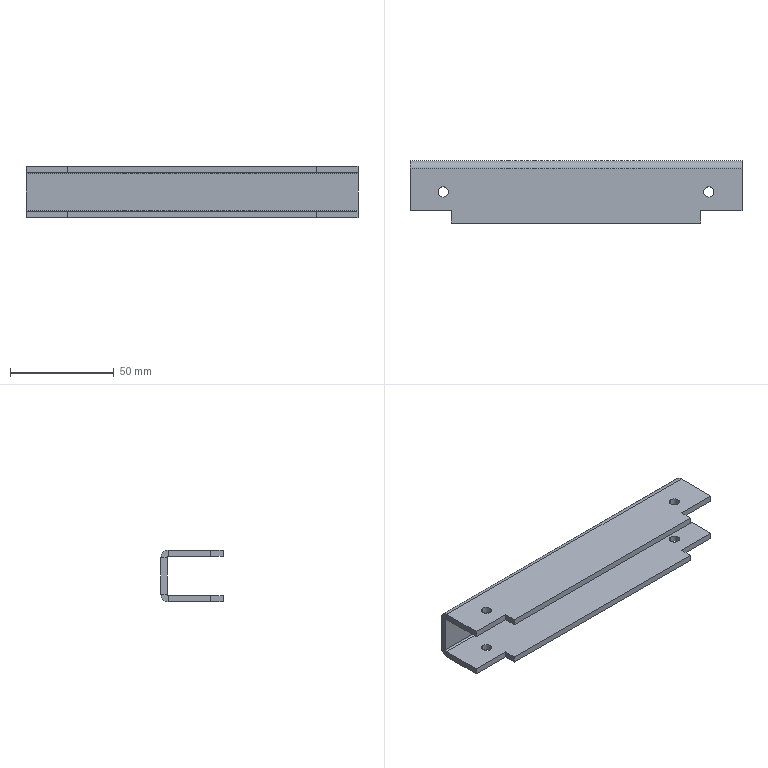Part | SolidWorks | features EdgeFlange 1, Fillet 1, FlatPattern 1, HoleWzd 1, ICE 1, SMBaseFlange 1, SheetMetal 1 | 1 solid | 38 faces | box 160 x 30 x 25 mm | volume 35323 mm3 | plane 26 | cylinder 12 | commonest cylinder face diameters 5 x8 1.473 x2 7.473 x2
STEP:
#1=CARTESIAN_POINT('',(64.,-17.5,12.5));
#2=VERTEX_POINT('',#1);
#3=CARTESIAN_POINT('',(64.,-12.5,12.5));
#4=VERTEX_POINT('',#3);
#5=CARTESIAN_POINT('',(64.,-15.,12.5));
#6=DIRECTION('',(0.,0.,-1.));
#7=DIRECTION('',(0.,1.,0.));
#8=AXIS2_PLACEMENT_3D('',#5,#6,#7);
#9=CIRCLE('',#8,2.5);
#10=EDGE_CURVE('',#2,#4,#9,.T.);
#11=ORIENTED_EDGE('',*,*,#10,.F.);
#12=CARTESIAN_POINT('',(64.,-17.5,9.5));
#13=VERTEX_POINT('',#12);
#14=CARTESIAN_POINT('',(64.,-17.5,-12.5));
#15=DIRECTION('',(0.,0.,-1.));
#16=VECTOR('',#15,1000.);
#17=LINE('',#14,#16);
#18=EDGE_CURVE('',#2,#13,#17,.T.);
#19=ORIENTED_EDGE('',*,*,#18,.T.);
#20=CARTESIAN_POINT('',(64.,-12.5,9.5));
#21=VERTEX_POINT('',#20);
#22=CARTESIAN_POINT('',(64.,-15.,9.5));
#23=DIRECTION('',(0.,0.,-1.));
#24=DIRECTION('',(0.,1.,0.));
#25=AXIS2_PLACEMENT_3D('',#22,#23,#24);
#26=CIRCLE('',#25,2.5);
#27=EDGE_CURVE('',#13,#21,#26,.T.);
#28=ORIENTED_EDGE('',*,*,#27,.T.);
#29=CARTESIAN_POINT('',(64.,-12.5,-12.5));
#30=DIRECTION('',(0.,0.,-1.));
#31=VECTOR('',#30,1000.);
#32=LINE('',#29,#31);
#33=EDGE_CURVE('',#4,#21,#32,.T.);
#34=ORIENTED_EDGE('',*,*,#33,.F.);
#35=EDGE_LOOP('',(#11,#19,#28,#34));
#36=FACE_OUTER_BOUND('',#35,.T.);
#37=CARTESIAN_POINT('',(64.,-15.,-12.5));
#38=DIRECTION('',(0.,0.,-1.));
#39=DIRECTION('',(0.,1.,0.));
#40=AXIS2_PLACEMENT_3D('',#37,#38,#39);
#41=CYLINDRICAL_SURFACE('',#40,2.5);
#42=ADVANCED_FACE('',(#36),#41,.F.);
#43=CARTESIAN_POINT('',(64.,-12.5,-9.5));
#44=VERTEX_POINT('',#43);
#45=CARTESIAN_POINT('',(64.,-17.5,-9.5));
#46=VERTEX_POINT('',#45);
#47=CARTESIAN_POINT('',(64.,-15.,-9.5));
#48=DIRECTION('',(0.,0.,1.));
#49=DIRECTION('',(0.,-1.,0.));
#50=AXIS2_PLACEMENT_3D('',#47,#48,#49);
#51=CIRCLE('',#50,2.5);
#52=EDGE_CURVE('',#44,#46,#51,.T.);
#53=ORIENTED_EDGE('',*,*,#52,.T.);
#54=CARTESIAN_POINT('',(64.,-17.5,-12.5));
#55=VERTEX_POINT('',#54);
#56=CARTESIAN_POINT('',(64.,-17.5,-12.5));
#57=DIRECTION('',(0.,0.,-1.));
#58=VECTOR('',#57,1000.);
#59=LINE('',#56,#58);
#60=EDGE_CURVE('',#46,#55,#59,.T.);
#61=ORIENTED_EDGE('',*,*,#60,.T.);
#62=CARTESIAN_POINT('',(64.,-12.5,-12.5));
#63=VERTEX_POINT('',#62);
#64=CARTESIAN_POINT('',(64.,-15.,-12.5));
#65=DIRECTION('',(0.,0.,-1.));
#66=DIRECTION('',(0.,1.,0.));
#67=AXIS2_PLACEMENT_3D('',#64,#65,#66);
#68=CIRCLE('',#67,2.5);
#69=EDGE_CURVE('',#55,#63,#68,.T.);
#70=ORIENTED_EDGE('',*,*,#69,.T.);
#71=CARTESIAN_POINT('',(64.,-12.5,-12.5));
#72=DIRECTION('',(0.,0.,-1.));
#73=VECTOR('',#72,1000.);
#74=LINE('',#71,#73);
#75=EDGE_CURVE('',#44,#63,#74,.T.);
#76=ORIENTED_EDGE('',*,*,#75,.F.);
#77=EDGE_LOOP('',(#53,#61,#70,#76));
#78=FACE_OUTER_BOUND('',#77,.T.);
#79=CARTESIAN_POINT('',(64.,-15.,-12.5));
#80=DIRECTION('',(0.,0.,-1.));
#81=DIRECTION('',(0.,1.,0.));
#82=AXIS2_PLACEMENT_3D('',#79,#80,#81);
#83=CYLINDRICAL_SURFACE('',#82,2.5);
#84=ADVANCED_FACE('',(#78),#83,.F.);
#85=CARTESIAN_POINT('',(-64.,-17.5,12.5));
#86=VERTEX_POINT('',#85);
#87=CARTESIAN_POINT('',(-64.,-12.5,12.5));
#88=VERTEX_POINT('',#87);
#89=CARTESIAN_POINT('',(-64.,-15.,12.5));
#90=DIRECTION('',(0.,0.,-1.));
#91=DIRECTION('',(0.,1.,0.));
#92=AXIS2_PLACEMENT_3D('',#89,#90,#91);
#93=CIRCLE('',#92,2.5);
#94=EDGE_CURVE('',#86,#88,#93,.T.);
#95=ORIENTED_EDGE('',*,*,#94,.F.);
#96=CARTESIAN_POINT('',(-64.,-17.5,9.5));
#97=VERTEX_POINT('',#96);
#98=CARTESIAN_POINT('',(-64.,-17.5,-12.5));
#99=DIRECTION('',(0.,0.,-1.));
#100=VECTOR('',#99,1000.);
#101=LINE('',#98,#100);
#102=EDGE_CURVE('',#86,#97,#101,.T.);
#103=ORIENTED_EDGE('',*,*,#102,.T.);
#104=CARTESIAN_POINT('',(-64.,-12.5,9.5));
#105=VERTEX_POINT('',#104);
#106=CARTESIAN_POINT('',(-64.,-15.,9.5));
#107=DIRECTION('',(0.,0.,-1.));
#108=DIRECTION('',(0.,1.,0.));
#109=AXIS2_PLACEMENT_3D('',#106,#107,#108);
#110=CIRCLE('',#109,2.5);
#111=EDGE_CURVE('',#97,#105,#110,.T.);
#112=ORIENTED_EDGE('',*,*,#111,.T.);
#113=CARTESIAN_POINT('',(-64.,-12.5,-12.5));
#114=DIRECTION('',(0.,0.,-1.));
#115=VECTOR('',#114,1000.);
#116=LINE('',#113,#115);
#117=EDGE_CURVE('',#88,#105,#116,.T.);
#118=ORIENTED_EDGE('',*,*,#117,.F.);
#119=EDGE_LOOP('',(#95,#103,#112,#118));
#120=FACE_OUTER_BOUND('',#119,.T.);
#121=CARTESIAN_POINT('',(-64.,-15.,-12.5));
#122=DIRECTION('',(0.,0.,-1.));
#123=DIRECTION('',(0.,1.,0.));
#124=AXIS2_PLACEMENT_3D('',#121,#122,#123);
#125=CYLINDRICAL_SURFACE('',#124,2.5);
#126=ADVANCED_FACE('',(#120),#125,.F.);
#127=CARTESIAN_POINT('',(-64.,-12.5,-9.5));
#128=VERTEX_POINT('',#127);
#129=CARTESIAN_POINT('',(-64.,-17.5,-9.5));
#130=VERTEX_POINT('',#129);
#131=CARTESIAN_POINT('',(-64.,-15.,-9.5));
#132=DIRECTION('',(0.,0.,1.));
#133=DIRECTION('',(0.,-1.,0.));
#134=AXIS2_PLACEMENT_3D('',#131,#132,#133);
#135=CIRCLE('',#134,2.5);
#136=EDGE_CURVE('',#128,#130,#135,.T.);
#137=ORIENTED_EDGE('',*,*,#136,.T.);
#138=CARTESIAN_POINT('',(-64.,-17.5,-12.5));
#139=VERTEX_POINT('',#138);
#140=CARTESIAN_POINT('',(-64.,-17.5,-12.5));
#141=DIRECTION('',(0.,0.,-1.));
#142=VECTOR('',#141,1000.);
#143=LINE('',#140,#142);
#144=EDGE_CURVE('',#130,#139,#143,.T.);
#145=ORIENTED_EDGE('',*,*,#144,.T.);
#146=CARTESIAN_POINT('',(-64.,-12.5,-12.5));
#147=VERTEX_POINT('',#146);
#148=CARTESIAN_POINT('',(-64.,-15.,-12.5));
#149=DIRECTION('',(0.,0.,-1.));
#150=DIRECTION('',(0.,1.,0.));
#151=AXIS2_PLACEMENT_3D('',#148,#149,#150);
#152=CIRCLE('',#151,2.5);
#153=EDGE_CURVE('',#139,#147,#152,.T.);
#154=ORIENTED_EDGE('',*,*,#153,.T.);
#155=CARTESIAN_POINT('',(-64.,-12.5,-12.5));
#156=DIRECTION('',(0.,0.,-1.));
#157=VECTOR('',#156,1000.);
#158=LINE('',#155,#157);
#159=EDGE_CURVE('',#128,#147,#158,.T.);
#160=ORIENTED_EDGE('',*,*,#159,.F.);
#161=EDGE_LOOP('',(#137,#145,#154,#160));
#162=FACE_OUTER_BOUND('',#161,.T.);
#163=CARTESIAN_POINT('',(-64.,-15.,-12.5));
#164=DIRECTION('',(0.,0.,-1.));
#165=DIRECTION('',(0.,1.,0.));
#166=AXIS2_PLACEMENT_3D('',#163,#164,#165);
#167=CYLINDRICAL_SURFACE('',#166,2.5);
#168=ADVANCED_FACE('',(#162),#167,.F.);
#169=CARTESIAN_POINT('',(80.,-3.,-8.763));
#170=VERTEX_POINT('',#169);
#171=CARTESIAN_POINT('',(-80.,-3.,-8.763));
#172=VERTEX_POINT('',#171);
#173=CARTESIAN_POINT('',(80.,-3.,-8.763));
#174=DIRECTION('',(-1.,0.,0.));
#175=VECTOR('',#174,1000.);
#176=LINE('',#173,#175);
#177=EDGE_CURVE('',#170,#172,#176,.T.);
#178=ORIENTED_EDGE('',*,*,#177,.F.);
#179=CARTESIAN_POINT('',(80.,-3.,8.763));
#180=VERTEX_POINT('',#179);
#181=CARTESIAN_POINT('',(80.,-3.,-12.5));
#182=DIRECTION('',(0.,0.,-1.));
#183=VECTOR('',#182,1000.);
#184=LINE('',#181,#183);
#185=EDGE_CURVE('',#180,#170,#184,.T.);
#186=ORIENTED_EDGE('',*,*,#185,.F.);
#187=CARTESIAN_POINT('',(-80.,-3.,8.763));
#188=VERTEX_POINT('',#187);
#189=CARTESIAN_POINT('',(-80.,-3.,8.763));
#190=DIRECTION('',(1.,0.,0.));
#191=VECTOR('',#190,1000.);
#192=LINE('',#189,#191);
#193=EDGE_CURVE('',#188,#180,#192,.T.);
#194=ORIENTED_EDGE('',*,*,#193,.F.);
#195=CARTESIAN_POINT('',(-80.,-3.,-12.5));
#196=DIRECTION('',(0.,0.,1.));
#197=VECTOR('',#196,1000.);
#198=LINE('',#195,#197);
#199=EDGE_CURVE('',#172,#188,#198,.T.);
#200=ORIENTED_EDGE('',*,*,#199,.F.);
#201=EDGE_LOOP('',(#178,#186,#194,#200));
#202=FACE_OUTER_BOUND('',#201,.T.);
#203=CARTESIAN_POINT('',(0.,-3.,0.));
#204=DIRECTION('',(0.,1.,0.));
#205=DIRECTION('',(0.,0.,1.));
#206=AXIS2_PLACEMENT_3D('',#203,#204,#205);
#207=PLANE('',#206);
#208=ADVANCED_FACE('',(#202),#207,.F.);
#209=CARTESIAN_POINT('',(80.,0.,8.763));
#210=VERTEX_POINT('',#209);
#211=CARTESIAN_POINT('',(80.,0.,-8.763));
#212=VERTEX_POINT('',#211);
#213=CARTESIAN_POINT('',(80.,0.,-12.5));
#214=DIRECTION('',(0.,0.,-1.));
#215=VECTOR('',#214,1000.);
#216=LINE('',#213,#215);
#217=EDGE_CURVE('',#210,#212,#216,.T.);
#218=ORIENTED_EDGE('',*,*,#217,.T.);
#219=CARTESIAN_POINT('',(-80.,0.,-8.763));
#220=VERTEX_POINT('',#219);
#221=CARTESIAN_POINT('',(80.,0.,-8.763));
#222=DIRECTION('',(-1.,0.,0.));
#223=VECTOR('',#222,1000.);
#224=LINE('',#221,#223);
#225=EDGE_CURVE('',#212,#220,#224,.T.);
#226=ORIENTED_EDGE('',*,*,#225,.T.);
#227=CARTESIAN_POINT('',(-80.,0.,8.763));
#228=VERTEX_POINT('',#227);
#229=CARTESIAN_POINT('',(-80.,0.,-12.5));
#230=DIRECTION('',(0.,0.,1.));
#231=VECTOR('',#230,1000.);
#232=LINE('',#229,#231);
#233=EDGE_CURVE('',#220,#228,#232,.T.);
#234=ORIENTED_EDGE('',*,*,#233,.T.);
#235=CARTESIAN_POINT('',(-80.,0.,8.763));
#236=DIRECTION('',(1.,0.,0.));
#237=VECTOR('',#236,1000.);
#238=LINE('',#235,#237);
#239=EDGE_CURVE('',#228,#210,#238,.T.);
#240=ORIENTED_EDGE('',*,*,#239,.T.);
#241=EDGE_LOOP('',(#218,#226,#234,#240));
#242=FACE_OUTER_BOUND('',#241,.T.);
#243=CARTESIAN_POINT('',(0.,0.,0.));
#244=DIRECTION('',(0.,1.,0.));
#245=DIRECTION('',(0.,0.,1.));
#246=AXIS2_PLACEMENT_3D('',#243,#244,#245);
#247=PLANE('',#246);
#248=ADVANCED_FACE('',(#242),#247,.T.);
#249=ORIENTED_EDGE('',*,*,#185,.T.);
#250=CARTESIAN_POINT('',(80.,-3.,-8.763));
#251=DIRECTION('',(0.,1.,0.));
#252=VECTOR('',#251,1000.);
#253=LINE('',#250,#252);
#254=EDGE_CURVE('',#170,#212,#253,.T.);
#255=ORIENTED_EDGE('',*,*,#254,.T.);
#256=ORIENTED_EDGE('',*,*,#217,.F.);
#257=CARTESIAN_POINT('',(80.,-3.,8.763));
#258=DIRECTION('',(0.,1.,0.));
#259=VECTOR('',#258,1000.);
#260=LINE('',#257,#259);
#261=EDGE_CURVE('',#180,#210,#260,.T.);
#262=ORIENTED_EDGE('',*,*,#261,.F.);
#263=EDGE_LOOP('',(#249,#255,#256,#262));
#264=FACE_OUTER_BOUND('',#263,.T.);
#265=CARTESIAN_POINT('',(80.,-3.,-12.5));
#266=DIRECTION('',(1.,0.,0.));
#267=DIRECTION('',(0.,0.,-1.));
#268=AXIS2_PLACEMENT_3D('',#265,#266,#267);
#269=PLANE('',#268);
#270=ADVANCED_FACE('',(#264),#269,.T.);
#271=CARTESIAN_POINT('',(-80.,-3.,-8.763));
#272=DIRECTION('',(0.,1.,0.));
#273=VECTOR('',#272,1000.);
#274=LINE('',#271,#273);
#275=EDGE_CURVE('',#172,#220,#274,.T.);
#276=ORIENTED_EDGE('',*,*,#275,.F.);
#277=ORIENTED_EDGE('',*,*,#199,.T.);
#278=CARTESIAN_POINT('',(-80.,-3.,8.763));
#279=DIRECTION('',(0.,1.,0.));
#280=VECTOR('',#279,1000.);
#281=LINE('',#278,#280);
#282=EDGE_CURVE('',#188,#228,#281,.T.);
#283=ORIENTED_EDGE('',*,*,#282,.T.);
#284=ORIENTED_EDGE('',*,*,#233,.F.);
#285=EDGE_LOOP('',(#276,#277,#283,#284));
#286=FACE_OUTER_BOUND('',#285,.T.);
#287=CARTESIAN_POINT('',(-80.,-3.,-12.5));
#288=DIRECTION('',(-1.,0.,0.));
#289=DIRECTION('',(0.,0.,1.));
#290=AXIS2_PLACEMENT_3D('',#287,#288,#289);
#291=PLANE('',#290);
#292=ADVANCED_FACE('',(#286),#291,.T.);
#293=CARTESIAN_POINT('',(80.,-3.737,9.5));
#294=VERTEX_POINT('',#293);
#295=CARTESIAN_POINT('',(80.,-3.737,12.5));
#296=VERTEX_POINT('',#295);
#297=CARTESIAN_POINT('',(80.,-3.737,12.5));
#298=DIRECTION('',(0.,0.,1.));
#299=VECTOR('',#298,1000.);
#300=LINE('',#297,#299);
#301=EDGE_CURVE('',#294,#296,#300,.T.);
#302=ORIENTED_EDGE('',*,*,#301,.F.);
#303=CARTESIAN_POINT('',(80.,-3.737,8.763));
#304=DIRECTION('',(1.,0.,0.));
#305=DIRECTION('',(0.,0.,1.));
#306=AXIS2_PLACEMENT_3D('',#303,#304,#305);
#307=CIRCLE('',#306,0.7366);
#308=EDGE_CURVE('',#180,#294,#307,.T.);
#309=ORIENTED_EDGE('',*,*,#308,.F.);
#310=ORIENTED_EDGE('',*,*,#261,.T.);
#311=CARTESIAN_POINT('',(80.,-3.737,8.763));
#312=DIRECTION('',(1.,0.,0.));
#313=DIRECTION('',(0.,0.,1.));
#314=AXIS2_PLACEMENT_3D('',#311,#312,#313);
#315=CIRCLE('',#314,3.737);
#316=EDGE_CURVE('',#210,#296,#315,.T.);
#317=ORIENTED_EDGE('',*,*,#316,.T.);
#318=EDGE_LOOP('',(#302,#309,#310,#317));
#319=FACE_OUTER_BOUND('',#318,.T.);
#320=CARTESIAN_POINT('',(80.,-3.737,8.763));
#321=DIRECTION('',(1.,0.,0.));
#322=DIRECTION('',(0.,0.,-1.));
#323=AXIS2_PLACEMENT_3D('',#320,#321,#322);
#324=PLANE('',#323);
#325=ADVANCED_FACE('',(#319),#324,.T.);
#326=CARTESIAN_POINT('',(-80.,-3.737,9.5));
#327=VERTEX_POINT('',#326);
#328=CARTESIAN_POINT('',(-80.,-3.737,8.763));
#329=DIRECTION('',(-1.,0.,0.));
#330=DIRECTION('',(0.,0.,1.));
#331=AXIS2_PLACEMENT_3D('',#328,#329,#330);
#332=CIRCLE('',#331,0.7366);
#333=EDGE_CURVE('',#327,#188,#332,.T.);
#334=ORIENTED_EDGE('',*,*,#333,.F.);
#335=CARTESIAN_POINT('',(-80.,-3.737,12.5));
#336=VERTEX_POINT('',#335);
#337=CARTESIAN_POINT('',(-80.,-3.737,9.5));
#338=DIRECTION('',(0.,0.,1.));
#339=VECTOR('',#338,1000.);
#340=LINE('',#337,#339);
#341=EDGE_CURVE('',#327,#336,#340,.T.);
#342=ORIENTED_EDGE('',*,*,#341,.T.);
#343=CARTESIAN_POINT('',(-80.,-3.737,8.763));
#344=DIRECTION('',(-1.,0.,0.));
#345=DIRECTION('',(0.,0.,1.));
#346=AXIS2_PLACEMENT_3D('',#343,#344,#345);
#347=CIRCLE('',#346,3.737);
#348=EDGE_CURVE('',#336,#228,#347,.T.);
#349=ORIENTED_EDGE('',*,*,#348,.T.);
#350=ORIENTED_EDGE('',*,*,#282,.F.);
#351=EDGE_LOOP('',(#334,#342,#349,#350));
#352=FACE_OUTER_BOUND('',#351,.T.);
#353=CARTESIAN_POINT('',(-80.,-3.737,8.763));
#354=DIRECTION('',(1.,0.,0.));
#355=DIRECTION('',(0.,0.,-1.));
#356=AXIS2_PLACEMENT_3D('',#353,#354,#355);
#357=PLANE('',#356);
#358=ADVANCED_FACE('',(#352),#357,.F.);
#359=ORIENTED_EDGE('',*,*,#239,.F.);
#360=ORIENTED_EDGE('',*,*,#348,.F.);
#361=CARTESIAN_POINT('',(80.,-3.737,12.5));
#362=DIRECTION('',(1.,0.,0.));
#363=VECTOR('',#362,1000.);
#364=LINE('',#361,#363);
#365=EDGE_CURVE('',#336,#296,#364,.T.);
#366=ORIENTED_EDGE('',*,*,#365,.T.);
#367=ORIENTED_EDGE('',*,*,#316,.F.);
#368=EDGE_LOOP('',(#359,#360,#366,#367));
#369=FACE_OUTER_BOUND('',#368,.T.);
#370=CARTESIAN_POINT('',(-80.,-3.737,8.763));
#371=DIRECTION('',(-1.,0.,0.));
#372=DIRECTION('',(0.,0.,1.));
#373=AXIS2_PLACEMENT_3D('',#370,#371,#372);
#374=CYLINDRICAL_SURFACE('',#373,3.737);
#375=ADVANCED_FACE('',(#369),#374,.T.);
#376=ORIENTED_EDGE('',*,*,#193,.T.);
#377=ORIENTED_EDGE('',*,*,#308,.T.);
#378=CARTESIAN_POINT('',(80.,-3.737,9.5));
#379=DIRECTION('',(-1.,0.,0.));
#380=VECTOR('',#379,1000.);
#381=LINE('',#378,#380);
#382=EDGE_CURVE('',#294,#327,#381,.T.);
#383=ORIENTED_EDGE('',*,*,#382,.T.);
#384=ORIENTED_EDGE('',*,*,#333,.T.);
#385=EDGE_LOOP('',(#376,#377,#383,#384));
#386=FACE_OUTER_BOUND('',#385,.T.);
#387=CARTESIAN_POINT('',(-80.,-3.737,8.763));
#388=DIRECTION('',(-1.,0.,0.));
#389=DIRECTION('',(0.,0.,1.));
#390=AXIS2_PLACEMENT_3D('',#387,#388,#389);
#391=CYLINDRICAL_SURFACE('',#390,0.7366);
#392=ADVANCED_FACE('',(#386),#391,.F.);
#393=CARTESIAN_POINT('',(-80.,-24.,9.5));
#394=VERTEX_POINT('',#393);
#395=CARTESIAN_POINT('',(-80.,-30.,9.5));
#396=DIRECTION('',(0.,-1.,0.));
#397=VECTOR('',#396,1000.);
#398=LINE('',#395,#397);
#399=EDGE_CURVE('',#327,#394,#398,.T.);
#400=ORIENTED_EDGE('',*,*,#399,.T.);
#401=CARTESIAN_POINT('',(-80.,-24.,12.5));
#402=VERTEX_POINT('',#401);
#403=CARTESIAN_POINT('',(-80.,-24.,12.5));
#404=DIRECTION('',(0.,0.,-1.));
#405=VECTOR('',#404,1000.);
#406=LINE('',#403,#405);
#407=EDGE_CURVE('',#402,#394,#406,.T.);
#408=ORIENTED_EDGE('',*,*,#407,.F.);
#409=CARTESIAN_POINT('',(-80.,0.,12.5));
#410=DIRECTION('',(0.,-1.,0.));
#411=VECTOR('',#410,1000.);
#412=LINE('',#409,#411);
#413=EDGE_CURVE('',#336,#402,#412,.T.);
#414=ORIENTED_EDGE('',*,*,#413,.F.);
#415=ORIENTED_EDGE('',*,*,#341,.F.);
#416=EDGE_LOOP('',(#400,#408,#414,#415));
#417=FACE_OUTER_BOUND('',#416,.T.);
#418=CARTESIAN_POINT('',(-80.,-30.,12.5));
#419=DIRECTION('',(1.,0.,0.));
#420=DIRECTION('',(0.,0.,-1.));
#421=AXIS2_PLACEMENT_3D('',#418,#419,#420);
#422=PLANE('',#421);
#423=ADVANCED_FACE('',(#417),#422,.F.);
#424=CARTESIAN_POINT('',(80.,-24.,12.5));
#425=VERTEX_POINT('',#424);
#426=CARTESIAN_POINT('',(80.,0.,12.5));
#427=DIRECTION('',(0.,1.,0.));
#428=VECTOR('',#427,1000.);
#429=LINE('',#426,#428);
#430=EDGE_CURVE('',#425,#296,#429,.T.);
#431=ORIENTED_EDGE('',*,*,#430,.F.);
#432=CARTESIAN_POINT('',(80.,-24.,9.5));
#433=VERTEX_POINT('',#432);
#434=CARTESIAN_POINT('',(80.,-24.,12.5));
#435=DIRECTION('',(0.,0.,-1.));
#436=VECTOR('',#435,1000.);
#437=LINE('',#434,#436);
#438=EDGE_CURVE('',#425,#433,#437,.T.);
#439=ORIENTED_EDGE('',*,*,#438,.T.);
#440=CARTESIAN_POINT('',(80.,-3.,9.5));
#441=DIRECTION('',(0.,1.,0.));
#442=VECTOR('',#441,1000.);
#443=LINE('',#440,#442);
#444=EDGE_CURVE('',#433,#294,#443,.T.);
#445=ORIENTED_EDGE('',*,*,#444,.T.);
#446=ORIENTED_EDGE('',*,*,#301,.T.);
#447=EDGE_LOOP('',(#431,#439,#445,#446));
#448=FACE_OUTER_BOUND('',#447,.T.);
#449=CARTESIAN_POINT('',(80.,-3.,12.5));
#450=DIRECTION('',(-1.,0.,0.));
#451=DIRECTION('',(0.,0.,1.));
#452=AXIS2_PLACEMENT_3D('',#449,#450,#451);
#453=PLANE('',#452);
#454=ADVANCED_FACE('',(#448),#453,.F.);
#455=CARTESIAN_POINT('',(64.,-15.,12.5));
#456=DIRECTION('',(0.,0.,-1.));
#457=DIRECTION('',(0.,1.,0.));
#458=AXIS2_PLACEMENT_3D('',#455,#456,#457);
#459=CIRCLE('',#458,2.5);
#460=EDGE_CURVE('',#4,#2,#459,.T.);
#461=ORIENTED_EDGE('',*,*,#460,.T.);
#462=ORIENTED_EDGE('',*,*,#10,.T.);
#463=EDGE_LOOP('',(#461,#462));
#464=FACE_BOUND('',#463,.T.);
#465=CARTESIAN_POINT('',(-64.,-15.,12.5));
#466=DIRECTION('',(0.,0.,-1.));
#467=DIRECTION('',(0.,1.,0.));
#468=AXIS2_PLACEMENT_3D('',#465,#466,#467);
#469=CIRCLE('',#468,2.5);
#470=EDGE_CURVE('',#88,#86,#469,.T.);
#471=ORIENTED_EDGE('',*,*,#470,.T.);
#472=ORIENTED_EDGE('',*,*,#94,.T.);
#473=EDGE_LOOP('',(#471,#472));
#474=FACE_BOUND('',#473,.T.);
#475=CARTESIAN_POINT('',(-60.,-24.,12.5));
#476=VERTEX_POINT('',#475);
#477=CARTESIAN_POINT('',(-80.,-24.,12.5));
#478=DIRECTION('',(1.,0.,0.));
#479=VECTOR('',#478,1000.);
#480=LINE('',#477,#479);
#481=EDGE_CURVE('',#402,#476,#480,.T.);
#482=ORIENTED_EDGE('',*,*,#481,.T.);
#483=CARTESIAN_POINT('',(-60.,-30.,12.5));
#484=VERTEX_POINT('',#483);
#485=CARTESIAN_POINT('',(-60.,-30.,12.5));
#486=DIRECTION('',(0.,-1.,0.));
#487=VECTOR('',#486,1000.);
#488=LINE('',#485,#487);
#489=EDGE_CURVE('',#476,#484,#488,.T.);
#490=ORIENTED_EDGE('',*,*,#489,.T.);
#491=CARTESIAN_POINT('',(60.,-30.,12.5));
#492=VERTEX_POINT('',#491);
#493=CARTESIAN_POINT('',(0.,-30.,12.5));
#494=DIRECTION('',(1.,0.,0.));
#495=VECTOR('',#494,1000.);
#496=LINE('',#493,#495);
#497=EDGE_CURVE('',#484,#492,#496,.T.);
#498=ORIENTED_EDGE('',*,*,#497,.T.);
#499=CARTESIAN_POINT('',(60.,-24.,12.5));
#500=VERTEX_POINT('',#499);
#501=CARTESIAN_POINT('',(60.,-30.,12.5));
#502=DIRECTION('',(0.,1.,0.));
#503=VECTOR('',#502,1000.);
#504=LINE('',#501,#503);
#505=EDGE_CURVE('',#492,#500,#504,.T.);
#506=ORIENTED_EDGE('',*,*,#505,.T.);
#507=CARTESIAN_POINT('',(80.,-24.,12.5));
#508=DIRECTION('',(1.,0.,0.));
#509=VECTOR('',#508,1000.);
#510=LINE('',#507,#509);
#511=EDGE_CURVE('',#500,#425,#510,.T.);
#512=ORIENTED_EDGE('',*,*,#511,.T.);
#513=ORIENTED_EDGE('',*,*,#430,.T.);
#514=ORIENTED_EDGE('',*,*,#365,.F.);
#515=ORIENTED_EDGE('',*,*,#413,.T.);
#516=EDGE_LOOP('',(#482,#490,#498,#506,#512,#513,#514,#515));
#517=FACE_OUTER_BOUND('',#516,.T.);
#518=CARTESIAN_POINT('',(0.,0.,12.5));
#519=DIRECTION('',(0.,0.,-1.));
#520=DIRECTION('',(0.,1.,0.));
#521=AXIS2_PLACEMENT_3D('',#518,#519,#520);
#522=PLANE('',#521);
#523=ADVANCED_FACE('',(#464,#474,#517),#522,.F.);
#524=CARTESIAN_POINT('',(64.,-15.,9.5));
#525=DIRECTION('',(0.,0.,-1.));
#526=DIRECTION('',(0.,1.,0.));
#527=AXIS2_PLACEMENT_3D('',#524,#525,#526);
#528=CIRCLE('',#527,2.5);
#529=EDGE_CURVE('',#21,#13,#528,.T.);
#530=ORIENTED_EDGE('',*,*,#529,.F.);
#531=ORIENTED_EDGE('',*,*,#27,.F.);
#532=EDGE_LOOP('',(#530,#531));
#533=FACE_BOUND('',#532,.T.);
#534=CARTESIAN_POINT('',(-64.,-15.,9.5));
#535=DIRECTION('',(0.,0.,-1.));
#536=DIRECTION('',(0.,1.,0.));
#537=AXIS2_PLACEMENT_3D('',#534,#535,#536);
#538=CIRCLE('',#537,2.5);
#539=EDGE_CURVE('',#105,#97,#538,.T.);
#540=ORIENTED_EDGE('',*,*,#539,.F.);
#541=ORIENTED_EDGE('',*,*,#111,.F.);
#542=EDGE_LOOP('',(#540,#541));
#543=FACE_BOUND('',#542,.T.);
#544=CARTESIAN_POINT('',(-60.,-24.,9.5));
#545=VERTEX_POINT('',#544);
#546=CARTESIAN_POINT('',(-60.,-30.,9.5));
#547=VERTEX_POINT('',#546);
#548=CARTESIAN_POINT('',(-60.,0.,9.5));
#549=DIRECTION('',(0.,-1.,0.));
#550=VECTOR('',#549,1000.);
#551=LINE('',#548,#550);
#552=EDGE_CURVE('',#545,#547,#551,.T.);
#553=ORIENTED_EDGE('',*,*,#552,.F.);
#554=CARTESIAN_POINT('',(0.,-24.,9.5));
#555=DIRECTION('',(1.,0.,0.));
#556=VECTOR('',#555,1000.);
#557=LINE('',#554,#556);
#558=EDGE_CURVE('',#394,#545,#557,.T.);
#559=ORIENTED_EDGE('',*,*,#558,.F.);
#560=ORIENTED_EDGE('',*,*,#399,.F.);
#561=ORIENTED_EDGE('',*,*,#382,.F.);
#562=ORIENTED_EDGE('',*,*,#444,.F.);
#563=CARTESIAN_POINT('',(60.,-24.,9.5));
#564=VERTEX_POINT('',#563);
#565=CARTESIAN_POINT('',(0.,-24.,9.5));
#566=DIRECTION('',(1.,0.,0.));
#567=VECTOR('',#566,1000.);
#568=LINE('',#565,#567);
#569=EDGE_CURVE('',#564,#433,#568,.T.);
#570=ORIENTED_EDGE('',*,*,#569,.F.);
#571=CARTESIAN_POINT('',(60.,-30.,9.5));
#572=VERTEX_POINT('',#571);
#573=CARTESIAN_POINT('',(60.,0.,9.5));
#574=DIRECTION('',(0.,1.,0.));
#575=VECTOR('',#574,1000.);
#576=LINE('',#573,#575);
#577=EDGE_CURVE('',#572,#564,#576,.T.);
#578=ORIENTED_EDGE('',*,*,#577,.F.);
#579=CARTESIAN_POINT('',(80.,-30.,9.5));
#580=DIRECTION('',(1.,0.,0.));
#581=VECTOR('',#580,1000.);
#582=LINE('',#579,#581);
#583=EDGE_CURVE('',#547,#572,#582,.T.);
#584=ORIENTED_EDGE('',*,*,#583,.F.);
#585=EDGE_LOOP('',(#553,#559,#560,#561,#562,#570,#578,#584));
#586=FACE_OUTER_BOUND('',#585,.T.);
#587=CARTESIAN_POINT('',(0.,0.,9.5));
#588=DIRECTION('',(0.,0.,-1.));
#589=DIRECTION('',(0.,1.,0.));
#590=AXIS2_PLACEMENT_3D('',#587,#588,#589);
#591=PLANE('',#590);
#592=ADVANCED_FACE('',(#533,#543,#586),#591,.T.);
#593=ORIENTED_EDGE('',*,*,#497,.F.);
#594=CARTESIAN_POINT('',(-60.,-30.,12.5));
#595=DIRECTION('',(0.,0.,-1.));
#596=VECTOR('',#595,1000.);
#597=LINE('',#594,#596);
#598=EDGE_CURVE('',#484,#547,#597,.T.);
#599=ORIENTED_EDGE('',*,*,#598,.T.);
#600=ORIENTED_EDGE('',*,*,#583,.T.);
#601=CARTESIAN_POINT('',(60.,-30.,12.5));
#602=DIRECTION('',(0.,0.,-1.));
#603=VECTOR('',#602,1000.);
#604=LINE('',#601,#603);
#605=EDGE_CURVE('',#492,#572,#604,.T.);
#606=ORIENTED_EDGE('',*,*,#605,.F.);
#607=EDGE_LOOP('',(#593,#599,#600,#606));
#608=FACE_OUTER_BOUND('',#607,.T.);
#609=CARTESIAN_POINT('',(80.,-30.,12.5));
#610=DIRECTION('',(0.,1.,0.));
#611=DIRECTION('',(0.,0.,1.));
#612=AXIS2_PLACEMENT_3D('',#609,#610,#611);
#613=PLANE('',#612);
#614=ADVANCED_FACE('',(#608),#613,.F.);
#615=CARTESIAN_POINT('',(-80.,-3.737,-9.5));
#616=VERTEX_POINT('',#615);
#617=CARTESIAN_POINT('',(-80.,-3.737,-12.5));
#618=VERTEX_POINT('',#617);
#619=CARTESIAN_POINT('',(-80.,-3.737,-12.5));
#620=DIRECTION('',(0.,0.,-1.));
#621=VECTOR('',#620,1000.);
#622=LINE('',#619,#621);
#623=EDGE_CURVE('',#616,#618,#622,.T.);
#624=ORIENTED_EDGE('',*,*,#623,.F.);
#625=CARTESIAN_POINT('',(-80.,-3.737,-8.763));
#626=DIRECTION('',(-1.,0.,0.));
#627=DIRECTION('',(0.,0.,-1.));
#628=AXIS2_PLACEMENT_3D('',#625,#626,#627);
#629=CIRCLE('',#628,0.7366);
#630=EDGE_CURVE('',#172,#616,#629,.T.);
#631=ORIENTED_EDGE('',*,*,#630,.F.);
#632=ORIENTED_EDGE('',*,*,#275,.T.);
#633=CARTESIAN_POINT('',(-80.,-3.737,-8.763));
#634=DIRECTION('',(-1.,0.,0.));
#635=DIRECTION('',(0.,0.,-1.));
#636=AXIS2_PLACEMENT_3D('',#633,#634,#635);
#637=CIRCLE('',#636,3.737);
#638=EDGE_CURVE('',#220,#618,#637,.T.);
#639=ORIENTED_EDGE('',*,*,#638,.T.);
#640=EDGE_LOOP('',(#624,#631,#632,#639));
#641=FACE_OUTER_BOUND('',#640,.T.);
#642=CARTESIAN_POINT('',(-80.,-3.737,-8.763));
#643=DIRECTION('',(-1.,0.,0.));
#644=DIRECTION('',(0.,0.,1.));
#645=AXIS2_PLACEMENT_3D('',#642,#643,#644);
#646=PLANE('',#645);
#647=ADVANCED_FACE('',(#641),#646,.T.);
#648=CARTESIAN_POINT('',(80.,-3.737,-9.5));
#649=VERTEX_POINT('',#648);
#650=CARTESIAN_POINT('',(80.,-3.737,-8.763));
#651=DIRECTION('',(1.,0.,0.));
#652=DIRECTION('',(0.,0.,-1.));
#653=AXIS2_PLACEMENT_3D('',#650,#651,#652);
#654=CIRCLE('',#653,0.7366);
#655=EDGE_CURVE('',#649,#170,#654,.T.);
#656=ORIENTED_EDGE('',*,*,#655,.F.);
#657=CARTESIAN_POINT('',(80.,-3.737,-12.5));
#658=VERTEX_POINT('',#657);
#659=CARTESIAN_POINT('',(80.,-3.737,-9.5));
#660=DIRECTION('',(0.,0.,-1.));
#661=VECTOR('',#660,1000.);
#662=LINE('',#659,#661);
#663=EDGE_CURVE('',#649,#658,#662,.T.);
#664=ORIENTED_EDGE('',*,*,#663,.T.);
#665=CARTESIAN_POINT('',(80.,-3.737,-8.763));
#666=DIRECTION('',(1.,0.,0.));
#667=DIRECTION('',(0.,0.,-1.));
#668=AXIS2_PLACEMENT_3D('',#665,#666,#667);
#669=CIRCLE('',#668,3.737);
#670=EDGE_CURVE('',#658,#212,#669,.T.);
#671=ORIENTED_EDGE('',*,*,#670,.T.);
#672=ORIENTED_EDGE('',*,*,#254,.F.);
#673=EDGE_LOOP('',(#656,#664,#671,#672));
#674=FACE_OUTER_BOUND('',#673,.T.);
#675=CARTESIAN_POINT('',(80.,-3.737,-8.763));
#676=DIRECTION('',(-1.,0.,0.));
#677=DIRECTION('',(0.,0.,1.));
#678=AXIS2_PLACEMENT_3D('',#675,#676,#677);
#679=PLANE('',#678);
#680=ADVANCED_FACE('',(#674),#679,.F.);
#681=ORIENTED_EDGE('',*,*,#225,.F.);
#682=ORIENTED_EDGE('',*,*,#670,.F.);
#683=CARTESIAN_POINT('',(-80.,-3.737,-12.5));
#684=DIRECTION('',(-1.,0.,0.));
#685=VECTOR('',#684,1000.);
#686=LINE('',#683,#685);
#687=EDGE_CURVE('',#658,#618,#686,.T.);
#688=ORIENTED_EDGE('',*,*,#687,.T.);
#689=ORIENTED_EDGE('',*,*,#638,.F.);
#690=EDGE_LOOP('',(#681,#682,#688,#689));
#691=FACE_OUTER_BOUND('',#690,.T.);
#692=CARTESIAN_POINT('',(80.,-3.737,-8.763));
#693=DIRECTION('',(1.,0.,0.));
#694=DIRECTION('',(0.,0.,-1.));
#695=AXIS2_PLACEMENT_3D('',#692,#693,#694);
#696=CYLINDRICAL_SURFACE('',#695,3.737);
#697=ADVANCED_FACE('',(#691),#696,.T.);
#698=ORIENTED_EDGE('',*,*,#177,.T.);
#699=ORIENTED_EDGE('',*,*,#630,.T.);
#700=CARTESIAN_POINT('',(-80.,-3.737,-9.5));
#701=DIRECTION('',(1.,0.,0.));
#702=VECTOR('',#701,1000.);
#703=LINE('',#700,#702);
#704=EDGE_CURVE('',#616,#649,#703,.T.);
#705=ORIENTED_EDGE('',*,*,#704,.T.);
#706=ORIENTED_EDGE('',*,*,#655,.T.);
#707=EDGE_LOOP('',(#698,#699,#705,#706));
#708=FACE_OUTER_BOUND('',#707,.T.);
#709=CARTESIAN_POINT('',(80.,-3.737,-8.763));
#710=DIRECTION('',(1.,0.,0.));
#711=DIRECTION('',(0.,0.,-1.));
#712=AXIS2_PLACEMENT_3D('',#709,#710,#711);
#713=CYLINDRICAL_SURFACE('',#712,0.7366);
#714=ADVANCED_FACE('',(#708),#713,.F.);
#715=CARTESIAN_POINT('',(80.,-24.,-9.5));
#716=VERTEX_POINT('',#715);
#717=CARTESIAN_POINT('',(80.,-30.,-9.5));
#718=DIRECTION('',(0.,-1.,0.));
#719=VECTOR('',#718,1000.);
#720=LINE('',#717,#719);
#721=EDGE_CURVE('',#649,#716,#720,.T.);
#722=ORIENTED_EDGE('',*,*,#721,.T.);
#723=CARTESIAN_POINT('',(80.,-24.,-12.5));
#724=VERTEX_POINT('',#723);
#725=CARTESIAN_POINT('',(80.,-24.,12.5));
#726=DIRECTION('',(0.,0.,-1.));
#727=VECTOR('',#726,1000.);
#728=LINE('',#725,#727);
#729=EDGE_CURVE('',#716,#724,#728,.T.);
#730=ORIENTED_EDGE('',*,*,#729,.T.);
#731=CARTESIAN_POINT('',(80.,0.,-12.5));
#732=DIRECTION('',(0.,-1.,0.));
#733=VECTOR('',#732,1000.);
#734=LINE('',#731,#733);
#735=EDGE_CURVE('',#658,#724,#734,.T.);
#736=ORIENTED_EDGE('',*,*,#735,.F.);
#737=ORIENTED_EDGE('',*,*,#663,.F.);
#738=EDGE_LOOP('',(#722,#730,#736,#737));
#739=FACE_OUTER_BOUND('',#738,.T.);
#740=CARTESIAN_POINT('',(80.,-30.,-12.5));
#741=DIRECTION('',(-1.,0.,0.));
#742=DIRECTION('',(0.,0.,1.));
#743=AXIS2_PLACEMENT_3D('',#740,#741,#742);
#744=PLANE('',#743);
#745=ADVANCED_FACE('',(#739),#744,.F.);
#746=CARTESIAN_POINT('',(-80.,-24.,-12.5));
#747=VERTEX_POINT('',#746);
#748=CARTESIAN_POINT('',(-80.,0.,-12.5));
#749=DIRECTION('',(0.,1.,0.));
#750=VECTOR('',#749,1000.);
#751=LINE('',#748,#750);
#752=EDGE_CURVE('',#747,#618,#751,.T.);
#753=ORIENTED_EDGE('',*,*,#752,.F.);
#754=CARTESIAN_POINT('',(-80.,-24.,-9.5));
#755=VERTEX_POINT('',#754);
#756=CARTESIAN_POINT('',(-80.,-24.,12.5));
#757=DIRECTION('',(0.,0.,-1.));
#758=VECTOR('',#757,1000.);
#759=LINE('',#756,#758);
#760=EDGE_CURVE('',#755,#747,#759,.T.);
#761=ORIENTED_EDGE('',*,*,#760,.F.);
#762=CARTESIAN_POINT('',(-80.,-3.,-9.5));
#763=DIRECTION('',(0.,1.,0.));
#764=VECTOR('',#763,1000.);
#765=LINE('',#762,#764);
#766=EDGE_CURVE('',#755,#616,#765,.T.);
#767=ORIENTED_EDGE('',*,*,#766,.T.);
#768=ORIENTED_EDGE('',*,*,#623,.T.);
#769=EDGE_LOOP('',(#753,#761,#767,#768));
#770=FACE_OUTER_BOUND('',#769,.T.);
#771=CARTESIAN_POINT('',(-80.,-3.,-12.5));
#772=DIRECTION('',(1.,0.,0.));
#773=DIRECTION('',(0.,0.,-1.));
#774=AXIS2_PLACEMENT_3D('',#771,#772,#773);
#775=PLANE('',#774);
#776=ADVANCED_FACE('',(#770),#775,.F.);
#777=CARTESIAN_POINT('',(64.,-15.,-12.5));
#778=DIRECTION('',(0.,0.,-1.));
#779=DIRECTION('',(0.,1.,0.));
#780=AXIS2_PLACEMENT_3D('',#777,#778,#779);
#781=CIRCLE('',#780,2.5);
#782=EDGE_CURVE('',#63,#55,#781,.T.);
#783=ORIENTED_EDGE('',*,*,#782,.F.);
#784=ORIENTED_EDGE('',*,*,#69,.F.);
#785=EDGE_LOOP('',(#783,#784));
#786=FACE_BOUND('',#785,.T.);
#787=CARTESIAN_POINT('',(-64.,-15.,-12.5));
#788=DIRECTION('',(0.,0.,-1.));
#789=DIRECTION('',(0.,1.,0.));
#790=AXIS2_PLACEMENT_3D('',#787,#788,#789);
#791=CIRCLE('',#790,2.5);
#792=EDGE_CURVE('',#147,#139,#791,.T.);
#793=ORIENTED_EDGE('',*,*,#792,.F.);
#794=ORIENTED_EDGE('',*,*,#153,.F.);
#795=EDGE_LOOP('',(#793,#794));
#796=FACE_BOUND('',#795,.T.);
#797=CARTESIAN_POINT('',(60.,-30.,-12.5));
#798=VERTEX_POINT('',#797);
#799=CARTESIAN_POINT('',(-60.,-30.,-12.5));
#800=VERTEX_POINT('',#799);
#801=CARTESIAN_POINT('',(0.,-30.,-12.5));
#802=DIRECTION('',(-1.,0.,0.));
#803=VECTOR('',#802,1000.);
#804=LINE('',#801,#803);
#805=EDGE_CURVE('',#798,#800,#804,.T.);
#806=ORIENTED_EDGE('',*,*,#805,.T.);
#807=CARTESIAN_POINT('',(-60.,-24.,-12.5));
#808=VERTEX_POINT('',#807);
#809=CARTESIAN_POINT('',(-60.,-30.,-12.5));
#810=DIRECTION('',(0.,-1.,0.));
#811=VECTOR('',#810,1000.);
#812=LINE('',#809,#811);
#813=EDGE_CURVE('',#808,#800,#812,.T.);
#814=ORIENTED_EDGE('',*,*,#813,.F.);
#815=CARTESIAN_POINT('',(-80.,-24.,-12.5));
#816=DIRECTION('',(1.,0.,0.));
#817=VECTOR('',#816,1000.);
#818=LINE('',#815,#817);
#819=EDGE_CURVE('',#747,#808,#818,.T.);
#820=ORIENTED_EDGE('',*,*,#819,.F.);
#821=ORIENTED_EDGE('',*,*,#752,.T.);
#822=ORIENTED_EDGE('',*,*,#687,.F.);
#823=ORIENTED_EDGE('',*,*,#735,.T.);
#824=CARTESIAN_POINT('',(60.,-24.,-12.5));
#825=VERTEX_POINT('',#824);
#826=CARTESIAN_POINT('',(80.,-24.,-12.5));
#827=DIRECTION('',(1.,0.,0.));
#828=VECTOR('',#827,1000.);
#829=LINE('',#826,#828);
#830=EDGE_CURVE('',#825,#724,#829,.T.);
#831=ORIENTED_EDGE('',*,*,#830,.F.);
#832=CARTESIAN_POINT('',(60.,-30.,-12.5));
#833=DIRECTION('',(0.,1.,0.));
#834=VECTOR('',#833,1000.);
#835=LINE('',#832,#834);
#836=EDGE_CURVE('',#798,#825,#835,.T.);
#837=ORIENTED_EDGE('',*,*,#836,.F.);
#838=EDGE_LOOP('',(#806,#814,#820,#821,#822,#823,#831,#837));
#839=FACE_OUTER_BOUND('',#838,.T.);
#840=CARTESIAN_POINT('',(0.,0.,-12.5));
#841=DIRECTION('',(0.,0.,1.));
#842=DIRECTION('',(0.,-1.,0.));
#843=AXIS2_PLACEMENT_3D('',#840,#841,#842);
#844=PLANE('',#843);
#845=ADVANCED_FACE('',(#786,#796,#839),#844,.F.);
#846=ORIENTED_EDGE('',*,*,#52,.F.);
#847=CARTESIAN_POINT('',(64.,-15.,-9.5));
#848=DIRECTION('',(0.,0.,1.));
#849=DIRECTION('',(0.,-1.,0.));
#850=AXIS2_PLACEMENT_3D('',#847,#848,#849);
#851=CIRCLE('',#850,2.5);
#852=EDGE_CURVE('',#46,#44,#851,.T.);
#853=ORIENTED_EDGE('',*,*,#852,.F.);
#854=EDGE_LOOP('',(#846,#853));
#855=FACE_BOUND('',#854,.T.);
#856=ORIENTED_EDGE('',*,*,#136,.F.);
#857=CARTESIAN_POINT('',(-64.,-15.,-9.5));
#858=DIRECTION('',(0.,0.,1.));
#859=DIRECTION('',(0.,-1.,0.));
#860=AXIS2_PLACEMENT_3D('',#857,#858,#859);
#861=CIRCLE('',#860,2.5);
#862=EDGE_CURVE('',#130,#128,#861,.T.);
#863=ORIENTED_EDGE('',*,*,#862,.F.);
#864=EDGE_LOOP('',(#856,#863));
#865=FACE_BOUND('',#864,.T.);
#866=CARTESIAN_POINT('',(-60.,-30.,-9.5));
#867=VERTEX_POINT('',#866);
#868=CARTESIAN_POINT('',(-60.,-24.,-9.5));
#869=VERTEX_POINT('',#868);
#870=CARTESIAN_POINT('',(-60.,0.,-9.5));
#871=DIRECTION('',(0.,1.,0.));
#872=VECTOR('',#871,1000.);
#873=LINE('',#870,#872);
#874=EDGE_CURVE('',#867,#869,#873,.T.);
#875=ORIENTED_EDGE('',*,*,#874,.F.);
#876=CARTESIAN_POINT('',(60.,-30.,-9.5));
#877=VERTEX_POINT('',#876);
#878=CARTESIAN_POINT('',(-80.,-30.,-9.5));
#879=DIRECTION('',(-1.,0.,0.));
#880=VECTOR('',#879,1000.);
#881=LINE('',#878,#880);
#882=EDGE_CURVE('',#877,#867,#881,.T.);
#883=ORIENTED_EDGE('',*,*,#882,.F.);
#884=CARTESIAN_POINT('',(60.,-24.,-9.5));
#885=VERTEX_POINT('',#884);
#886=CARTESIAN_POINT('',(60.,0.,-9.5));
#887=DIRECTION('',(0.,-1.,0.));
#888=VECTOR('',#887,1000.);
#889=LINE('',#886,#888);
#890=EDGE_CURVE('',#885,#877,#889,.T.);
#891=ORIENTED_EDGE('',*,*,#890,.F.);
#892=CARTESIAN_POINT('',(0.,-24.,-9.5));
#893=DIRECTION('',(-1.,0.,0.));
#894=VECTOR('',#893,1000.);
#895=LINE('',#892,#894);
#896=EDGE_CURVE('',#716,#885,#895,.T.);
#897=ORIENTED_EDGE('',*,*,#896,.F.);
#898=ORIENTED_EDGE('',*,*,#721,.F.);
#899=ORIENTED_EDGE('',*,*,#704,.F.);
#900=ORIENTED_EDGE('',*,*,#766,.F.);
#901=CARTESIAN_POINT('',(0.,-24.,-9.5));
#902=DIRECTION('',(-1.,0.,0.));
#903=VECTOR('',#902,1000.);
#904=LINE('',#901,#903);
#905=EDGE_CURVE('',#869,#755,#904,.T.);
#906=ORIENTED_EDGE('',*,*,#905,.F.);
#907=EDGE_LOOP('',(#875,#883,#891,#897,#898,#899,#900,#906));
#908=FACE_OUTER_BOUND('',#907,.T.);
#909=CARTESIAN_POINT('',(0.,0.,-9.5));
#910=DIRECTION('',(0.,0.,1.));
#911=DIRECTION('',(0.,-1.,0.));
#912=AXIS2_PLACEMENT_3D('',#909,#910,#911);
#913=PLANE('',#912);
#914=ADVANCED_FACE('',(#855,#865,#908),#913,.T.);
#915=ORIENTED_EDGE('',*,*,#882,.T.);
#916=CARTESIAN_POINT('',(-60.,-30.,-12.5));
#917=DIRECTION('',(0.,0.,-1.));
#918=VECTOR('',#917,1000.);
#919=LINE('',#916,#918);
#920=EDGE_CURVE('',#867,#800,#919,.T.);
#921=ORIENTED_EDGE('',*,*,#920,.T.);
#922=ORIENTED_EDGE('',*,*,#805,.F.);
#923=CARTESIAN_POINT('',(60.,-30.,-12.5));
#924=DIRECTION('',(0.,0.,1.));
#925=VECTOR('',#924,1000.);
#926=LINE('',#923,#925);
#927=EDGE_CURVE('',#798,#877,#926,.T.);
#928=ORIENTED_EDGE('',*,*,#927,.T.);
#929=EDGE_LOOP('',(#915,#921,#922,#928));
#930=FACE_OUTER_BOUND('',#929,.T.);
#931=CARTESIAN_POINT('',(-80.,-30.,-12.5));
#932=DIRECTION('',(0.,1.,0.));
#933=DIRECTION('',(0.,0.,1.));
#934=AXIS2_PLACEMENT_3D('',#931,#932,#933);
#935=PLANE('',#934);
#936=ADVANCED_FACE('',(#930),#935,.F.);
#937=ORIENTED_EDGE('',*,*,#890,.T.);
#938=ORIENTED_EDGE('',*,*,#927,.F.);
#939=ORIENTED_EDGE('',*,*,#836,.T.);
#940=CARTESIAN_POINT('',(60.,-24.,12.5));
#941=DIRECTION('',(0.,0.,-1.));
#942=VECTOR('',#941,1000.);
#943=LINE('',#940,#942);
#944=EDGE_CURVE('',#885,#825,#943,.T.);
#945=ORIENTED_EDGE('',*,*,#944,.F.);
#946=EDGE_LOOP('',(#937,#938,#939,#945));
#947=FACE_OUTER_BOUND('',#946,.T.);
#948=CARTESIAN_POINT('',(60.,-30.,12.5));
#949=DIRECTION('',(-1.,0.,0.));
#950=DIRECTION('',(0.,0.,1.));
#951=AXIS2_PLACEMENT_3D('',#948,#949,#950);
#952=PLANE('',#951);
#953=ADVANCED_FACE('',(#947),#952,.F.);
#954=ORIENTED_EDGE('',*,*,#896,.T.);
#955=ORIENTED_EDGE('',*,*,#944,.T.);
#956=ORIENTED_EDGE('',*,*,#830,.T.);
#957=ORIENTED_EDGE('',*,*,#729,.F.);
#958=EDGE_LOOP('',(#954,#955,#956,#957));
#959=FACE_OUTER_BOUND('',#958,.T.);
#960=CARTESIAN_POINT('',(80.,-24.,12.5));
#961=DIRECTION('',(0.,1.,0.));
#962=DIRECTION('',(0.,0.,1.));
#963=AXIS2_PLACEMENT_3D('',#960,#961,#962);
#964=PLANE('',#963);
#965=ADVANCED_FACE('',(#959),#964,.F.);
#966=ORIENTED_EDGE('',*,*,#569,.T.);
#967=ORIENTED_EDGE('',*,*,#438,.F.);
#968=ORIENTED_EDGE('',*,*,#511,.F.);
#969=CARTESIAN_POINT('',(60.,-24.,12.5));
#970=DIRECTION('',(0.,0.,-1.));
#971=VECTOR('',#970,1000.);
#972=LINE('',#969,#971);
#973=EDGE_CURVE('',#500,#564,#972,.T.);
#974=ORIENTED_EDGE('',*,*,#973,.T.);
#975=EDGE_LOOP('',(#966,#967,#968,#974));
#976=FACE_OUTER_BOUND('',#975,.T.);
#977=CARTESIAN_POINT('',(80.,-24.,12.5));
#978=DIRECTION('',(0.,1.,0.));
#979=DIRECTION('',(0.,0.,1.));
#980=AXIS2_PLACEMENT_3D('',#977,#978,#979);
#981=PLANE('',#980);
#982=ADVANCED_FACE('',(#976),#981,.F.);
#983=ORIENTED_EDGE('',*,*,#577,.T.);
#984=ORIENTED_EDGE('',*,*,#973,.F.);
#985=ORIENTED_EDGE('',*,*,#505,.F.);
#986=ORIENTED_EDGE('',*,*,#605,.T.);
#987=EDGE_LOOP('',(#983,#984,#985,#986));
#988=FACE_OUTER_BOUND('',#987,.T.);
#989=CARTESIAN_POINT('',(60.,-30.,12.5));
#990=DIRECTION('',(-1.,0.,0.));
#991=DIRECTION('',(0.,0.,1.));
#992=AXIS2_PLACEMENT_3D('',#989,#990,#991);
#993=PLANE('',#992);
#994=ADVANCED_FACE('',(#988),#993,.F.);
#995=ORIENTED_EDGE('',*,*,#874,.T.);
#996=CARTESIAN_POINT('',(-60.,-24.,12.5));
#997=DIRECTION('',(0.,0.,-1.));
#998=VECTOR('',#997,1000.);
#999=LINE('',#996,#998);
#1000=EDGE_CURVE('',#869,#808,#999,.T.);
#1001=ORIENTED_EDGE('',*,*,#1000,.T.);
#1002=ORIENTED_EDGE('',*,*,#813,.T.);
#1003=ORIENTED_EDGE('',*,*,#920,.F.);
#1004=EDGE_LOOP('',(#995,#1001,#1002,#1003));
#1005=FACE_OUTER_BOUND('',#1004,.T.);
#1006=CARTESIAN_POINT('',(-60.,-30.,12.5));
#1007=DIRECTION('',(1.,0.,0.));
#1008=DIRECTION('',(0.,1.,0.));
#1009=AXIS2_PLACEMENT_3D('',#1006,#1007,#1008);
#1010=PLANE('',#1009);
#1011=ADVANCED_FACE('',(#1005),#1010,.F.);
#1012=ORIENTED_EDGE('',*,*,#905,.T.);
#1013=ORIENTED_EDGE('',*,*,#760,.T.);
#1014=ORIENTED_EDGE('',*,*,#819,.T.);
#1015=ORIENTED_EDGE('',*,*,#1000,.F.);
#1016=EDGE_LOOP('',(#1012,#1013,#1014,#1015));
#1017=FACE_OUTER_BOUND('',#1016,.T.);
#1018=CARTESIAN_POINT('',(-80.,-24.,12.5));
#1019=DIRECTION('',(0.,1.,0.));
#1020=DIRECTION('',(0.,0.,1.));
#1021=AXIS2_PLACEMENT_3D('',#1018,#1019,#1020);
#1022=PLANE('',#1021);
#1023=ADVANCED_FACE('',(#1017),#1022,.F.);
#1024=ORIENTED_EDGE('',*,*,#558,.T.);
#1025=CARTESIAN_POINT('',(-60.,-24.,12.5));
#1026=DIRECTION('',(0.,0.,-1.));
#1027=VECTOR('',#1026,1000.);
#1028=LINE('',#1025,#1027);
#1029=EDGE_CURVE('',#476,#545,#1028,.T.);
#1030=ORIENTED_EDGE('',*,*,#1029,.F.);
#1031=ORIENTED_EDGE('',*,*,#481,.F.);
#1032=ORIENTED_EDGE('',*,*,#407,.T.);
#1033=EDGE_LOOP('',(#1024,#1030,#1031,#1032));
#1034=FACE_OUTER_BOUND('',#1033,.T.);
#1035=CARTESIAN_POINT('',(-80.,-24.,12.5));
#1036=DIRECTION('',(0.,1.,0.));
#1037=DIRECTION('',(0.,0.,1.));
#1038=AXIS2_PLACEMENT_3D('',#1035,#1036,#1037);
#1039=PLANE('',#1038);
#1040=ADVANCED_FACE('',(#1034),#1039,.F.);
#1041=ORIENTED_EDGE('',*,*,#552,.T.);
#1042=ORIENTED_EDGE('',*,*,#598,.F.);
#1043=ORIENTED_EDGE('',*,*,#489,.F.);
#1044=ORIENTED_EDGE('',*,*,#1029,.T.);
#1045=EDGE_LOOP('',(#1041,#1042,#1043,#1044));
#1046=FACE_OUTER_BOUND('',#1045,.T.);
#1047=CARTESIAN_POINT('',(-60.,-30.,12.5));
#1048=DIRECTION('',(1.,0.,0.));
#1049=DIRECTION('',(0.,1.,0.));
#1050=AXIS2_PLACEMENT_3D('',#1047,#1048,#1049);
#1051=PLANE('',#1050);
#1052=ADVANCED_FACE('',(#1046),#1051,.F.);
#1053=ORIENTED_EDGE('',*,*,#144,.F.);
#1054=ORIENTED_EDGE('',*,*,#862,.T.);
#1055=ORIENTED_EDGE('',*,*,#159,.T.);
#1056=ORIENTED_EDGE('',*,*,#792,.T.);
#1057=EDGE_LOOP('',(#1053,#1054,#1055,#1056));
#1058=FACE_OUTER_BOUND('',#1057,.T.);
#1059=CARTESIAN_POINT('',(-64.,-15.,-12.5));
#1060=DIRECTION('',(0.,0.,-1.));
#1061=DIRECTION('',(0.,1.,0.));
#1062=AXIS2_PLACEMENT_3D('',#1059,#1060,#1061);
#1063=CYLINDRICAL_SURFACE('',#1062,2.5);
#1064=ADVANCED_FACE('',(#1058),#1063,.F.);
#1065=ORIENTED_EDGE('',*,*,#102,.F.);
#1066=ORIENTED_EDGE('',*,*,#470,.F.);
#1067=ORIENTED_EDGE('',*,*,#117,.T.);
#1068=ORIENTED_EDGE('',*,*,#539,.T.);
#1069=EDGE_LOOP('',(#1065,#1066,#1067,#1068));
#1070=FACE_OUTER_BOUND('',#1069,.T.);
#1071=CARTESIAN_POINT('',(-64.,-15.,-12.5));
#1072=DIRECTION('',(0.,0.,-1.));
#1073=DIRECTION('',(0.,1.,0.));
#1074=AXIS2_PLACEMENT_3D('',#1071,#1072,#1073);
#1075=CYLINDRICAL_SURFACE('',#1074,2.5);
#1076=ADVANCED_FACE('',(#1070),#1075,.F.);
#1077=ORIENTED_EDGE('',*,*,#60,.F.);
#1078=ORIENTED_EDGE('',*,*,#852,.T.);
#1079=ORIENTED_EDGE('',*,*,#75,.T.);
#1080=ORIENTED_EDGE('',*,*,#782,.T.);
#1081=EDGE_LOOP('',(#1077,#1078,#1079,#1080));
#1082=FACE_OUTER_BOUND('',#1081,.T.);
#1083=CARTESIAN_POINT('',(64.,-15.,-12.5));
#1084=DIRECTION('',(0.,0.,-1.));
#1085=DIRECTION('',(0.,1.,0.));
#1086=AXIS2_PLACEMENT_3D('',#1083,#1084,#1085);
#1087=CYLINDRICAL_SURFACE('',#1086,2.5);
#1088=ADVANCED_FACE('',(#1082),#1087,.F.);
#1089=ORIENTED_EDGE('',*,*,#18,.F.);
#1090=ORIENTED_EDGE('',*,*,#460,.F.);
#1091=ORIENTED_EDGE('',*,*,#33,.T.);
#1092=ORIENTED_EDGE('',*,*,#529,.T.);
#1093=EDGE_LOOP('',(#1089,#1090,#1091,#1092));
#1094=FACE_OUTER_BOUND('',#1093,.T.);
#1095=CARTESIAN_POINT('',(64.,-15.,-12.5));
#1096=DIRECTION('',(0.,0.,-1.));
#1097=DIRECTION('',(0.,1.,0.));
#1098=AXIS2_PLACEMENT_3D('',#1095,#1096,#1097);
#1099=CYLINDRICAL_SURFACE('',#1098,2.5);
#1100=ADVANCED_FACE('',(#1094),#1099,.F.);
#1101=CLOSED_SHELL('',(#42,#84,#126,#168,#208,#248,#270,#292,#325,#358,#375,#392,#423,#454,#523,#592,#614,#647,#680,#697,#714,#745,#776,#845,#914,#936,#953,#965,#982,#994,#1011,#1023,#1040,#1052,#1064,#1076,#1088,#1100));
#1102=MANIFOLD_SOLID_BREP('',#1101);
#1103=CARTESIAN_POINT('',(0.,0.,0.));
#1104=DIRECTION('',(0.,0.,1.));
#1105=DIRECTION('',(1.,0.,0.));
#1106=AXIS2_PLACEMENT_3D('',#1103,#1104,#1105);
#1107=(LENGTH_UNIT()NAMED_UNIT(*)SI_UNIT(.MILLI.,.METRE.));
#1108=UNCERTAINTY_MEASURE_WITH_UNIT(LENGTH_MEASURE(0.00001),#1107,'','');
#1109=(NAMED_UNIT(*)PLANE_ANGLE_UNIT()SI_UNIT($,.RADIAN.));
#1110=(NAMED_UNIT(*)SI_UNIT($,.STERADIAN.)SOLID_ANGLE_UNIT());
#1111=(GEOMETRIC_REPRESENTATION_CONTEXT(3)GLOBAL_UNCERTAINTY_ASSIGNED_CONTEXT((#1108))GLOBAL_UNIT_ASSIGNED_CONTEXT((#1107,#1109,#1110))REPRESENTATION_CONTEXT('',''));
#1112=ADVANCED_BREP_SHAPE_REPRESENTATION('',(#1102,#1106),#1111);